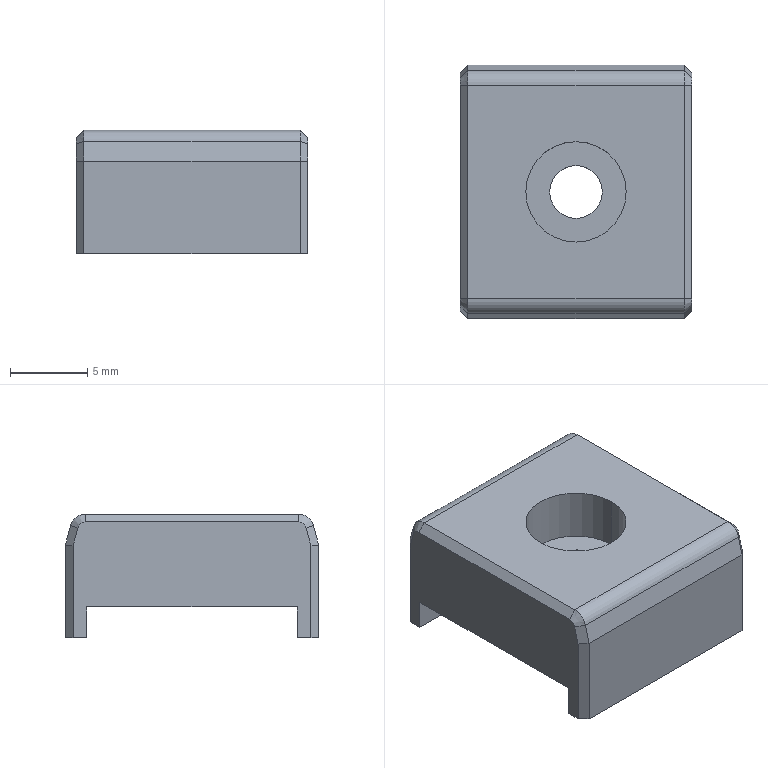Part | SolidWorks | features Chamfer 1, Extrusion 1, HoleWzd 1 | 1 solid | 33 faces | box 15 x 16.4 x 8 mm | volume 1396 mm3 | plane 23 | cylinder 6 | cone 4 | commonest cylinder face diameters 2 x2 3.4 x2 6.5 x2
STEP:
#1=CARTESIAN_POINT('',(-3.25,0.,-3.4));
#2=VERTEX_POINT('',#1);
#3=CARTESIAN_POINT('',(3.25,0.,-3.4));
#4=VERTEX_POINT('',#3);
#5=CARTESIAN_POINT('',(0.,0.,-3.4));
#6=DIRECTION('',(0.,0.,1.));
#7=DIRECTION('',(1.,0.,0.));
#8=AXIS2_PLACEMENT_3D('',#5,#6,#7);
#9=CIRCLE('',#8,3.25);
#10=EDGE_CURVE('',#2,#4,#9,.T.);
#11=ORIENTED_EDGE('',*,*,#10,.F.);
#12=CARTESIAN_POINT('',(-3.25,0.,0.));
#13=VERTEX_POINT('',#12);
#14=CARTESIAN_POINT('',(-3.25,0.,0.));
#15=DIRECTION('',(0.,0.,1.));
#16=VECTOR('',#15,1000.);
#17=LINE('',#14,#16);
#18=EDGE_CURVE('',#2,#13,#17,.T.);
#19=ORIENTED_EDGE('',*,*,#18,.T.);
#20=CARTESIAN_POINT('',(3.25,0.,0.));
#21=VERTEX_POINT('',#20);
#22=CARTESIAN_POINT('',(0.,0.,0.));
#23=DIRECTION('',(0.,0.,1.));
#24=DIRECTION('',(1.,0.,0.));
#25=AXIS2_PLACEMENT_3D('',#22,#23,#24);
#26=CIRCLE('',#25,3.25);
#27=EDGE_CURVE('',#13,#21,#26,.T.);
#28=ORIENTED_EDGE('',*,*,#27,.T.);
#29=CARTESIAN_POINT('',(3.25,0.,0.));
#30=DIRECTION('',(0.,0.,1.));
#31=VECTOR('',#30,1000.);
#32=LINE('',#29,#31);
#33=EDGE_CURVE('',#4,#21,#32,.T.);
#34=ORIENTED_EDGE('',*,*,#33,.F.);
#35=EDGE_LOOP('',(#11,#19,#28,#34));
#36=FACE_OUTER_BOUND('',#35,.T.);
#37=CARTESIAN_POINT('',(0.,0.,0.));
#38=DIRECTION('',(0.,0.,1.));
#39=DIRECTION('',(1.,0.,0.));
#40=AXIS2_PLACEMENT_3D('',#37,#38,#39);
#41=CYLINDRICAL_SURFACE('',#40,3.25);
#42=ADVANCED_FACE('',(#36),#41,.F.);
#43=CARTESIAN_POINT('',(1.7,0.,-6.));
#44=VERTEX_POINT('',#43);
#45=CARTESIAN_POINT('',(-1.7,0.,-6.));
#46=VERTEX_POINT('',#45);
#47=CARTESIAN_POINT('',(0.,0.,-6.));
#48=DIRECTION('',(0.,0.,-1.));
#49=DIRECTION('',(-1.,0.,0.));
#50=AXIS2_PLACEMENT_3D('',#47,#48,#49);
#51=CIRCLE('',#50,1.7);
#52=EDGE_CURVE('',#44,#46,#51,.T.);
#53=ORIENTED_EDGE('',*,*,#52,.T.);
#54=CARTESIAN_POINT('',(-1.7,0.,-3.4));
#55=VERTEX_POINT('',#54);
#56=CARTESIAN_POINT('',(-1.7,0.,0.));
#57=DIRECTION('',(0.,0.,1.));
#58=VECTOR('',#57,1000.);
#59=LINE('',#56,#58);
#60=EDGE_CURVE('',#46,#55,#59,.T.);
#61=ORIENTED_EDGE('',*,*,#60,.T.);
#62=CARTESIAN_POINT('',(1.7,0.,-3.4));
#63=VERTEX_POINT('',#62);
#64=CARTESIAN_POINT('',(0.,0.,-3.4));
#65=DIRECTION('',(0.,0.,1.));
#66=DIRECTION('',(1.,0.,0.));
#67=AXIS2_PLACEMENT_3D('',#64,#65,#66);
#68=CIRCLE('',#67,1.7);
#69=EDGE_CURVE('',#55,#63,#68,.T.);
#70=ORIENTED_EDGE('',*,*,#69,.T.);
#71=CARTESIAN_POINT('',(1.7,0.,0.));
#72=DIRECTION('',(0.,0.,1.));
#73=VECTOR('',#72,1000.);
#74=LINE('',#71,#73);
#75=EDGE_CURVE('',#44,#63,#74,.T.);
#76=ORIENTED_EDGE('',*,*,#75,.F.);
#77=EDGE_LOOP('',(#53,#61,#70,#76));
#78=FACE_OUTER_BOUND('',#77,.T.);
#79=CARTESIAN_POINT('',(0.,0.,0.));
#80=DIRECTION('',(0.,0.,1.));
#81=DIRECTION('',(1.,0.,0.));
#82=AXIS2_PLACEMENT_3D('',#79,#80,#81);
#83=CYLINDRICAL_SURFACE('',#82,1.7);
#84=ADVANCED_FACE('',(#78),#83,.F.);
#85=ORIENTED_EDGE('',*,*,#52,.F.);
#86=CARTESIAN_POINT('',(0.,0.,-6.));
#87=DIRECTION('',(0.,0.,-1.));
#88=DIRECTION('',(-1.,0.,0.));
#89=AXIS2_PLACEMENT_3D('',#86,#87,#88);
#90=CIRCLE('',#89,1.7);
#91=EDGE_CURVE('',#46,#44,#90,.T.);
#92=ORIENTED_EDGE('',*,*,#91,.F.);
#93=EDGE_LOOP('',(#85,#92));
#94=FACE_BOUND('',#93,.T.);
#95=CARTESIAN_POINT('',(7.5,-6.8,-6.));
#96=VERTEX_POINT('',#95);
#97=CARTESIAN_POINT('',(7.5,6.8,-6.));
#98=VERTEX_POINT('',#97);
#99=CARTESIAN_POINT('',(7.5,6.8,-6.));
#100=DIRECTION('',(0.,1.,0.));
#101=VECTOR('',#100,1000.);
#102=LINE('',#99,#101);
#103=EDGE_CURVE('',#96,#98,#102,.T.);
#104=ORIENTED_EDGE('',*,*,#103,.F.);
#105=CARTESIAN_POINT('',(-7.5,-6.8,-6.));
#106=VERTEX_POINT('',#105);
#107=CARTESIAN_POINT('',(25.747,-6.8,-6.));
#108=DIRECTION('',(-1.,0.,0.));
#109=VECTOR('',#108,1000.);
#110=LINE('',#107,#109);
#111=EDGE_CURVE('',#96,#106,#110,.T.);
#112=ORIENTED_EDGE('',*,*,#111,.T.);
#113=CARTESIAN_POINT('',(-7.5,6.8,-6.));
#114=VERTEX_POINT('',#113);
#115=CARTESIAN_POINT('',(-7.5,6.8,-6.));
#116=DIRECTION('',(0.,-1.,0.));
#117=VECTOR('',#116,1000.);
#118=LINE('',#115,#117);
#119=EDGE_CURVE('',#114,#106,#118,.T.);
#120=ORIENTED_EDGE('',*,*,#119,.F.);
#121=CARTESIAN_POINT('',(25.747,6.8,-6.));
#122=DIRECTION('',(-1.,0.,0.));
#123=VECTOR('',#122,1000.);
#124=LINE('',#121,#123);
#125=EDGE_CURVE('',#98,#114,#124,.T.);
#126=ORIENTED_EDGE('',*,*,#125,.F.);
#127=EDGE_LOOP('',(#104,#112,#120,#126));
#128=FACE_OUTER_BOUND('',#127,.T.);
#129=CARTESIAN_POINT('',(25.747,6.8,-6.));
#130=DIRECTION('',(0.,0.,-1.));
#131=DIRECTION('',(-1.,0.,0.));
#132=AXIS2_PLACEMENT_3D('',#129,#130,#131);
#133=PLANE('',#132);
#134=ADVANCED_FACE('',(#94,#128),#133,.T.);
#135=CARTESIAN_POINT('',(7.5,6.8,-8.));
#136=VERTEX_POINT('',#135);
#137=CARTESIAN_POINT('',(7.5,6.8,-6.));
#138=DIRECTION('',(0.,0.,-1.));
#139=VECTOR('',#138,1000.);
#140=LINE('',#137,#139);
#141=EDGE_CURVE('',#98,#136,#140,.T.);
#142=ORIENTED_EDGE('',*,*,#141,.F.);
#143=ORIENTED_EDGE('',*,*,#125,.T.);
#144=CARTESIAN_POINT('',(-7.5,6.8,-8.));
#145=VERTEX_POINT('',#144);
#146=CARTESIAN_POINT('',(-7.5,6.8,-6.));
#147=DIRECTION('',(0.,0.,1.));
#148=VECTOR('',#147,1000.);
#149=LINE('',#146,#148);
#150=EDGE_CURVE('',#145,#114,#149,.T.);
#151=ORIENTED_EDGE('',*,*,#150,.F.);
#152=CARTESIAN_POINT('',(25.747,6.8,-8.));
#153=DIRECTION('',(-1.,0.,0.));
#154=VECTOR('',#153,1000.);
#155=LINE('',#152,#154);
#156=EDGE_CURVE('',#136,#145,#155,.T.);
#157=ORIENTED_EDGE('',*,*,#156,.F.);
#158=EDGE_LOOP('',(#142,#143,#151,#157));
#159=FACE_OUTER_BOUND('',#158,.T.);
#160=CARTESIAN_POINT('',(25.747,6.8,-6.));
#161=DIRECTION('',(0.,-1.,0.));
#162=DIRECTION('',(0.,0.,-1.));
#163=AXIS2_PLACEMENT_3D('',#160,#161,#162);
#164=PLANE('',#163);
#165=ADVANCED_FACE('',(#159),#164,.T.);
#166=CARTESIAN_POINT('',(-7.5,7.7,-8.));
#167=VERTEX_POINT('',#166);
#168=CARTESIAN_POINT('',(-7.5,6.8,-8.));
#169=DIRECTION('',(0.,-1.,0.));
#170=VECTOR('',#169,1000.);
#171=LINE('',#168,#170);
#172=EDGE_CURVE('',#167,#145,#171,.T.);
#173=ORIENTED_EDGE('',*,*,#172,.F.);
#174=CARTESIAN_POINT('',(-7.,8.2,-8.));
#175=VERTEX_POINT('',#174);
#176=CARTESIAN_POINT('',(8.674,23.874,-8.));
#177=DIRECTION('',(0.7071,0.7071,0.));
#178=VECTOR('',#177,1000.);
#179=LINE('',#176,#178);
#180=EDGE_CURVE('',#167,#175,#179,.T.);
#181=ORIENTED_EDGE('',*,*,#180,.T.);
#182=CARTESIAN_POINT('',(7.,8.2,-8.));
#183=VERTEX_POINT('',#182);
#184=CARTESIAN_POINT('',(25.747,8.2,-8.));
#185=DIRECTION('',(-1.,0.,0.));
#186=VECTOR('',#185,1000.);
#187=LINE('',#184,#186);
#188=EDGE_CURVE('',#183,#175,#187,.T.);
#189=ORIENTED_EDGE('',*,*,#188,.F.);
#190=CARTESIAN_POINT('',(7.5,7.7,-8.));
#191=VERTEX_POINT('',#190);
#192=CARTESIAN_POINT('',(17.074,-1.874,-8.));
#193=DIRECTION('',(0.7071,-0.7071,0.));
#194=VECTOR('',#193,1000.);
#195=LINE('',#192,#194);
#196=EDGE_CURVE('',#183,#191,#195,.T.);
#197=ORIENTED_EDGE('',*,*,#196,.T.);
#198=CARTESIAN_POINT('',(7.5,6.8,-8.));
#199=DIRECTION('',(0.,1.,0.));
#200=VECTOR('',#199,1000.);
#201=LINE('',#198,#200);
#202=EDGE_CURVE('',#136,#191,#201,.T.);
#203=ORIENTED_EDGE('',*,*,#202,.F.);
#204=ORIENTED_EDGE('',*,*,#156,.T.);
#205=EDGE_LOOP('',(#173,#181,#189,#197,#203,#204));
#206=FACE_OUTER_BOUND('',#205,.T.);
#207=CARTESIAN_POINT('',(25.747,6.8,-8.));
#208=DIRECTION('',(0.,0.,-1.));
#209=DIRECTION('',(-1.,0.,0.));
#210=AXIS2_PLACEMENT_3D('',#207,#208,#209);
#211=PLANE('',#210);
#212=ADVANCED_FACE('',(#206),#211,.T.);
#213=ORIENTED_EDGE('',*,*,#188,.T.);
#214=CARTESIAN_POINT('',(-7.,8.2,-2.));
#215=VERTEX_POINT('',#214);
#216=CARTESIAN_POINT('',(-7.,8.2,-8.));
#217=DIRECTION('',(0.,0.,1.));
#218=VECTOR('',#217,1000.);
#219=LINE('',#216,#218);
#220=EDGE_CURVE('',#175,#215,#219,.T.);
#221=ORIENTED_EDGE('',*,*,#220,.T.);
#222=CARTESIAN_POINT('',(7.,8.2,-2.));
#223=VERTEX_POINT('',#222);
#224=CARTESIAN_POINT('',(25.747,8.2,-2.));
#225=DIRECTION('',(-1.,0.,0.));
#226=VECTOR('',#225,1000.);
#227=LINE('',#224,#226);
#228=EDGE_CURVE('',#223,#215,#227,.T.);
#229=ORIENTED_EDGE('',*,*,#228,.F.);
#230=CARTESIAN_POINT('',(7.,8.2,-8.));
#231=DIRECTION('',(0.,0.,-1.));
#232=VECTOR('',#231,1000.);
#233=LINE('',#230,#232);
#234=EDGE_CURVE('',#223,#183,#233,.T.);
#235=ORIENTED_EDGE('',*,*,#234,.T.);
#236=EDGE_LOOP('',(#213,#221,#229,#235));
#237=FACE_OUTER_BOUND('',#236,.T.);
#238=CARTESIAN_POINT('',(25.747,8.2,-8.));
#239=DIRECTION('',(0.,1.,0.));
#240=DIRECTION('',(0.,0.,1.));
#241=AXIS2_PLACEMENT_3D('',#238,#239,#240);
#242=PLANE('',#241);
#243=ADVANCED_FACE('',(#237),#242,.T.);
#244=ORIENTED_EDGE('',*,*,#228,.T.);
#245=CARTESIAN_POINT('',(-7.,7.863,-0.7412));
#246=VERTEX_POINT('',#245);
#247=CARTESIAN_POINT('',(-7.,8.2,-2.));
#248=DIRECTION('',(0.,-0.2588,0.9659));
#249=VECTOR('',#248,1000.);
#250=LINE('',#247,#249);
#251=EDGE_CURVE('',#215,#246,#250,.T.);
#252=ORIENTED_EDGE('',*,*,#251,.T.);
#253=CARTESIAN_POINT('',(7.,7.863,-0.7412));
#254=VERTEX_POINT('',#253);
#255=CARTESIAN_POINT('',(25.747,7.863,-0.7412));
#256=DIRECTION('',(-1.,0.,0.));
#257=VECTOR('',#256,1000.);
#258=LINE('',#255,#257);
#259=EDGE_CURVE('',#254,#246,#258,.T.);
#260=ORIENTED_EDGE('',*,*,#259,.F.);
#261=CARTESIAN_POINT('',(7.,8.2,-2.));
#262=DIRECTION('',(0.,0.2588,-0.9659));
#263=VECTOR('',#262,1000.);
#264=LINE('',#261,#263);
#265=EDGE_CURVE('',#254,#223,#264,.T.);
#266=ORIENTED_EDGE('',*,*,#265,.T.);
#267=EDGE_LOOP('',(#244,#252,#260,#266));
#268=FACE_OUTER_BOUND('',#267,.T.);
#269=CARTESIAN_POINT('',(25.747,8.2,-2.));
#270=DIRECTION('',(0.,0.9659,0.2588));
#271=DIRECTION('',(0.,-0.2588,0.9659));
#272=AXIS2_PLACEMENT_3D('',#269,#270,#271);
#273=PLANE('',#272);
#274=ADVANCED_FACE('',(#268),#273,.T.);
#275=ORIENTED_EDGE('',*,*,#259,.T.);
#276=CARTESIAN_POINT('',(-7.,6.897,0.));
#277=VERTEX_POINT('',#276);
#278=CARTESIAN_POINT('',(-7.,6.897,-1.));
#279=DIRECTION('',(1.,0.,0.));
#280=DIRECTION('',(0.,0.,1.));
#281=AXIS2_PLACEMENT_3D('',#278,#279,#280);
#282=CIRCLE('',#281,1.);
#283=EDGE_CURVE('',#246,#277,#282,.T.);
#284=ORIENTED_EDGE('',*,*,#283,.T.);
#285=CARTESIAN_POINT('',(7.,6.897,0.));
#286=VERTEX_POINT('',#285);
#287=CARTESIAN_POINT('',(25.747,6.897,0.));
#288=DIRECTION('',(-1.,0.,0.));
#289=VECTOR('',#288,1000.);
#290=LINE('',#287,#289);
#291=EDGE_CURVE('',#286,#277,#290,.T.);
#292=ORIENTED_EDGE('',*,*,#291,.F.);
#293=CARTESIAN_POINT('',(7.,6.897,-1.));
#294=DIRECTION('',(-1.,0.,0.));
#295=DIRECTION('',(0.,0.,1.));
#296=AXIS2_PLACEMENT_3D('',#293,#294,#295);
#297=CIRCLE('',#296,1.);
#298=EDGE_CURVE('',#286,#254,#297,.T.);
#299=ORIENTED_EDGE('',*,*,#298,.T.);
#300=EDGE_LOOP('',(#275,#284,#292,#299));
#301=FACE_OUTER_BOUND('',#300,.T.);
#302=CARTESIAN_POINT('',(25.747,6.897,-1.));
#303=DIRECTION('',(-1.,0.,0.));
#304=DIRECTION('',(0.,0.,1.));
#305=AXIS2_PLACEMENT_3D('',#302,#303,#304);
#306=CYLINDRICAL_SURFACE('',#305,1.);
#307=ADVANCED_FACE('',(#301),#306,.T.);
#308=CARTESIAN_POINT('',(0.,0.,0.));
#309=DIRECTION('',(0.,0.,1.));
#310=DIRECTION('',(1.,0.,0.));
#311=AXIS2_PLACEMENT_3D('',#308,#309,#310);
#312=CIRCLE('',#311,3.25);
#313=EDGE_CURVE('',#21,#13,#312,.T.);
#314=ORIENTED_EDGE('',*,*,#313,.F.);
#315=ORIENTED_EDGE('',*,*,#27,.F.);
#316=EDGE_LOOP('',(#314,#315));
#317=FACE_BOUND('',#316,.T.);
#318=ORIENTED_EDGE('',*,*,#291,.T.);
#319=CARTESIAN_POINT('',(-7.,-6.897,0.));
#320=VERTEX_POINT('',#319);
#321=CARTESIAN_POINT('',(-7.,-6.897,0.));
#322=DIRECTION('',(0.,-1.,0.));
#323=VECTOR('',#322,1000.);
#324=LINE('',#321,#323);
#325=EDGE_CURVE('',#277,#320,#324,.T.);
#326=ORIENTED_EDGE('',*,*,#325,.T.);
#327=CARTESIAN_POINT('',(7.,-6.897,0.));
#328=VERTEX_POINT('',#327);
#329=CARTESIAN_POINT('',(25.747,-6.897,0.));
#330=DIRECTION('',(-1.,0.,0.));
#331=VECTOR('',#330,1000.);
#332=LINE('',#329,#331);
#333=EDGE_CURVE('',#328,#320,#332,.T.);
#334=ORIENTED_EDGE('',*,*,#333,.F.);
#335=CARTESIAN_POINT('',(7.,6.897,0.));
#336=DIRECTION('',(0.,1.,0.));
#337=VECTOR('',#336,1000.);
#338=LINE('',#335,#337);
#339=EDGE_CURVE('',#328,#286,#338,.T.);
#340=ORIENTED_EDGE('',*,*,#339,.T.);
#341=EDGE_LOOP('',(#318,#326,#334,#340));
#342=FACE_OUTER_BOUND('',#341,.T.);
#343=CARTESIAN_POINT('',(25.747,-6.897,0.));
#344=DIRECTION('',(0.,0.,1.));
#345=DIRECTION('',(1.,0.,0.));
#346=AXIS2_PLACEMENT_3D('',#343,#344,#345);
#347=PLANE('',#346);
#348=ADVANCED_FACE('',(#317,#342),#347,.T.);
#349=ORIENTED_EDGE('',*,*,#333,.T.);
#350=CARTESIAN_POINT('',(-7.,-7.863,-0.7412));
#351=VERTEX_POINT('',#350);
#352=CARTESIAN_POINT('',(-7.,-6.897,-1.));
#353=DIRECTION('',(1.,0.,0.));
#354=DIRECTION('',(0.,0.,1.));
#355=AXIS2_PLACEMENT_3D('',#352,#353,#354);
#356=CIRCLE('',#355,1.);
#357=EDGE_CURVE('',#320,#351,#356,.T.);
#358=ORIENTED_EDGE('',*,*,#357,.T.);
#359=CARTESIAN_POINT('',(7.,-7.863,-0.7412));
#360=VERTEX_POINT('',#359);
#361=CARTESIAN_POINT('',(25.747,-7.863,-0.7412));
#362=DIRECTION('',(-1.,0.,0.));
#363=VECTOR('',#362,1000.);
#364=LINE('',#361,#363);
#365=EDGE_CURVE('',#360,#351,#364,.T.);
#366=ORIENTED_EDGE('',*,*,#365,.F.);
#367=CARTESIAN_POINT('',(7.,-6.897,-1.));
#368=DIRECTION('',(-1.,0.,0.));
#369=DIRECTION('',(0.,0.,1.));
#370=AXIS2_PLACEMENT_3D('',#367,#368,#369);
#371=CIRCLE('',#370,1.);
#372=EDGE_CURVE('',#360,#328,#371,.T.);
#373=ORIENTED_EDGE('',*,*,#372,.T.);
#374=EDGE_LOOP('',(#349,#358,#366,#373));
#375=FACE_OUTER_BOUND('',#374,.T.);
#376=CARTESIAN_POINT('',(25.747,-6.897,-1.));
#377=DIRECTION('',(-1.,0.,0.));
#378=DIRECTION('',(0.,0.,1.));
#379=AXIS2_PLACEMENT_3D('',#376,#377,#378);
#380=CYLINDRICAL_SURFACE('',#379,1.);
#381=ADVANCED_FACE('',(#375),#380,.T.);
#382=ORIENTED_EDGE('',*,*,#365,.T.);
#383=CARTESIAN_POINT('',(-7.,-8.2,-2.));
#384=VERTEX_POINT('',#383);
#385=CARTESIAN_POINT('',(-7.,-8.2,-2.));
#386=DIRECTION('',(0.,-0.2588,-0.9659));
#387=VECTOR('',#386,1000.);
#388=LINE('',#385,#387);
#389=EDGE_CURVE('',#351,#384,#388,.T.);
#390=ORIENTED_EDGE('',*,*,#389,.T.);
#391=CARTESIAN_POINT('',(7.,-8.2,-2.));
#392=VERTEX_POINT('',#391);
#393=CARTESIAN_POINT('',(25.747,-8.2,-2.));
#394=DIRECTION('',(-1.,0.,0.));
#395=VECTOR('',#394,1000.);
#396=LINE('',#393,#395);
#397=EDGE_CURVE('',#392,#384,#396,.T.);
#398=ORIENTED_EDGE('',*,*,#397,.F.);
#399=CARTESIAN_POINT('',(7.,-7.863,-0.7412));
#400=DIRECTION('',(0.,0.2588,0.9659));
#401=VECTOR('',#400,1000.);
#402=LINE('',#399,#401);
#403=EDGE_CURVE('',#392,#360,#402,.T.);
#404=ORIENTED_EDGE('',*,*,#403,.T.);
#405=EDGE_LOOP('',(#382,#390,#398,#404));
#406=FACE_OUTER_BOUND('',#405,.T.);
#407=CARTESIAN_POINT('',(25.747,-8.2,-2.));
#408=DIRECTION('',(0.,-0.9659,0.2588));
#409=DIRECTION('',(0.,-0.2588,-0.9659));
#410=AXIS2_PLACEMENT_3D('',#407,#408,#409);
#411=PLANE('',#410);
#412=ADVANCED_FACE('',(#406),#411,.T.);
#413=CARTESIAN_POINT('',(7.,-8.2,-8.));
#414=VERTEX_POINT('',#413);
#415=CARTESIAN_POINT('',(-7.,-8.2,-8.));
#416=VERTEX_POINT('',#415);
#417=CARTESIAN_POINT('',(25.747,-8.2,-8.));
#418=DIRECTION('',(-1.,0.,0.));
#419=VECTOR('',#418,1000.);
#420=LINE('',#417,#419);
#421=EDGE_CURVE('',#414,#416,#420,.T.);
#422=ORIENTED_EDGE('',*,*,#421,.F.);
#423=CARTESIAN_POINT('',(7.,-8.2,-2.));
#424=DIRECTION('',(0.,0.,1.));
#425=VECTOR('',#424,1000.);
#426=LINE('',#423,#425);
#427=EDGE_CURVE('',#414,#392,#426,.T.);
#428=ORIENTED_EDGE('',*,*,#427,.T.);
#429=ORIENTED_EDGE('',*,*,#397,.T.);
#430=CARTESIAN_POINT('',(-7.,-8.2,-8.));
#431=DIRECTION('',(0.,0.,-1.));
#432=VECTOR('',#431,1000.);
#433=LINE('',#430,#432);
#434=EDGE_CURVE('',#384,#416,#433,.T.);
#435=ORIENTED_EDGE('',*,*,#434,.T.);
#436=EDGE_LOOP('',(#422,#428,#429,#435));
#437=FACE_OUTER_BOUND('',#436,.T.);
#438=CARTESIAN_POINT('',(25.747,-8.2,-8.));
#439=DIRECTION('',(0.,-1.,0.));
#440=DIRECTION('',(0.,0.,-1.));
#441=AXIS2_PLACEMENT_3D('',#438,#439,#440);
#442=PLANE('',#441);
#443=ADVANCED_FACE('',(#437),#442,.T.);
#444=CARTESIAN_POINT('',(7.5,-7.7,-8.));
#445=VERTEX_POINT('',#444);
#446=CARTESIAN_POINT('',(7.5,-6.8,-8.));
#447=VERTEX_POINT('',#446);
#448=CARTESIAN_POINT('',(7.5,-6.8,-8.));
#449=DIRECTION('',(0.,1.,0.));
#450=VECTOR('',#449,1000.);
#451=LINE('',#448,#450);
#452=EDGE_CURVE('',#445,#447,#451,.T.);
#453=ORIENTED_EDGE('',*,*,#452,.F.);
#454=CARTESIAN_POINT('',(17.074,1.874,-8.));
#455=DIRECTION('',(-0.7071,-0.7071,0.));
#456=VECTOR('',#455,1000.);
#457=LINE('',#454,#456);
#458=EDGE_CURVE('',#445,#414,#457,.T.);
#459=ORIENTED_EDGE('',*,*,#458,.T.);
#460=ORIENTED_EDGE('',*,*,#421,.T.);
#461=CARTESIAN_POINT('',(-7.5,-7.7,-8.));
#462=VERTEX_POINT('',#461);
#463=CARTESIAN_POINT('',(8.674,-23.874,-8.));
#464=DIRECTION('',(-0.7071,0.7071,0.));
#465=VECTOR('',#464,1000.);
#466=LINE('',#463,#465);
#467=EDGE_CURVE('',#416,#462,#466,.T.);
#468=ORIENTED_EDGE('',*,*,#467,.T.);
#469=CARTESIAN_POINT('',(-7.5,-6.8,-8.));
#470=VERTEX_POINT('',#469);
#471=CARTESIAN_POINT('',(-7.5,-6.8,-8.));
#472=DIRECTION('',(0.,-1.,0.));
#473=VECTOR('',#472,1000.);
#474=LINE('',#471,#473);
#475=EDGE_CURVE('',#470,#462,#474,.T.);
#476=ORIENTED_EDGE('',*,*,#475,.F.);
#477=CARTESIAN_POINT('',(25.747,-6.8,-8.));
#478=DIRECTION('',(-1.,0.,0.));
#479=VECTOR('',#478,1000.);
#480=LINE('',#477,#479);
#481=EDGE_CURVE('',#447,#470,#480,.T.);
#482=ORIENTED_EDGE('',*,*,#481,.F.);
#483=EDGE_LOOP('',(#453,#459,#460,#468,#476,#482));
#484=FACE_OUTER_BOUND('',#483,.T.);
#485=CARTESIAN_POINT('',(25.747,-6.8,-8.));
#486=DIRECTION('',(0.,0.,-1.));
#487=DIRECTION('',(-1.,0.,0.));
#488=AXIS2_PLACEMENT_3D('',#485,#486,#487);
#489=PLANE('',#488);
#490=ADVANCED_FACE('',(#484),#489,.T.);
#491=CARTESIAN_POINT('',(7.5,-6.8,-6.));
#492=DIRECTION('',(0.,0.,1.));
#493=VECTOR('',#492,1000.);
#494=LINE('',#491,#493);
#495=EDGE_CURVE('',#447,#96,#494,.T.);
#496=ORIENTED_EDGE('',*,*,#495,.F.);
#497=ORIENTED_EDGE('',*,*,#481,.T.);
#498=CARTESIAN_POINT('',(-7.5,-6.8,-6.));
#499=DIRECTION('',(0.,0.,-1.));
#500=VECTOR('',#499,1000.);
#501=LINE('',#498,#500);
#502=EDGE_CURVE('',#106,#470,#501,.T.);
#503=ORIENTED_EDGE('',*,*,#502,.F.);
#504=ORIENTED_EDGE('',*,*,#111,.F.);
#505=EDGE_LOOP('',(#496,#497,#503,#504));
#506=FACE_OUTER_BOUND('',#505,.T.);
#507=CARTESIAN_POINT('',(25.747,-6.8,-6.));
#508=DIRECTION('',(0.,1.,0.));
#509=DIRECTION('',(0.,0.,1.));
#510=AXIS2_PLACEMENT_3D('',#507,#508,#509);
#511=PLANE('',#510);
#512=ADVANCED_FACE('',(#506),#511,.T.);
#513=CARTESIAN_POINT('',(-7.5,7.38,-0.8706));
#514=VERTEX_POINT('',#513);
#515=CARTESIAN_POINT('',(-7.5,7.7,-2.066));
#516=VERTEX_POINT('',#515);
#517=CARTESIAN_POINT('',(-7.5,6.456,2.578));
#518=DIRECTION('',(0.,0.2588,-0.9659));
#519=VECTOR('',#518,1000.);
#520=LINE('',#517,#519);
#521=EDGE_CURVE('',#514,#516,#520,.T.);
#522=ORIENTED_EDGE('',*,*,#521,.T.);
#523=CARTESIAN_POINT('',(-7.5,7.7,-1.));
#524=DIRECTION('',(0.,0.,-1.));
#525=VECTOR('',#524,1000.);
#526=LINE('',#523,#525);
#527=EDGE_CURVE('',#516,#167,#526,.T.);
#528=ORIENTED_EDGE('',*,*,#527,.T.);
#529=ORIENTED_EDGE('',*,*,#172,.T.);
#530=ORIENTED_EDGE('',*,*,#150,.T.);
#531=ORIENTED_EDGE('',*,*,#119,.T.);
#532=ORIENTED_EDGE('',*,*,#502,.T.);
#533=ORIENTED_EDGE('',*,*,#475,.T.);
#534=CARTESIAN_POINT('',(-7.5,-7.7,-2.066));
#535=VERTEX_POINT('',#534);
#536=CARTESIAN_POINT('',(-7.5,-7.7,-1.));
#537=DIRECTION('',(0.,0.,1.));
#538=VECTOR('',#537,1000.);
#539=LINE('',#536,#538);
#540=EDGE_CURVE('',#462,#535,#539,.T.);
#541=ORIENTED_EDGE('',*,*,#540,.T.);
#542=CARTESIAN_POINT('',(-7.5,-7.38,-0.8706));
#543=VERTEX_POINT('',#542);
#544=CARTESIAN_POINT('',(-7.5,-7.38,-0.8706));
#545=DIRECTION('',(0.,0.2588,0.9659));
#546=VECTOR('',#545,1000.);
#547=LINE('',#544,#546);
#548=EDGE_CURVE('',#535,#543,#547,.T.);
#549=ORIENTED_EDGE('',*,*,#548,.T.);
#550=CARTESIAN_POINT('',(-7.5,-6.897,-0.5));
#551=VERTEX_POINT('',#550);
#552=CARTESIAN_POINT('',(-7.5,-6.897,-1.));
#553=DIRECTION('',(-1.,0.,0.));
#554=DIRECTION('',(0.,0.,1.));
#555=AXIS2_PLACEMENT_3D('',#552,#553,#554);
#556=CIRCLE('',#555,0.5);
#557=EDGE_CURVE('',#543,#551,#556,.T.);
#558=ORIENTED_EDGE('',*,*,#557,.T.);
#559=CARTESIAN_POINT('',(-7.5,6.897,-0.5));
#560=VERTEX_POINT('',#559);
#561=CARTESIAN_POINT('',(-7.5,-6.897,-0.5));
#562=DIRECTION('',(0.,1.,0.));
#563=VECTOR('',#562,1000.);
#564=LINE('',#561,#563);
#565=EDGE_CURVE('',#551,#560,#564,.T.);
#566=ORIENTED_EDGE('',*,*,#565,.T.);
#567=CARTESIAN_POINT('',(-7.5,6.897,-1.));
#568=DIRECTION('',(-1.,0.,0.));
#569=DIRECTION('',(0.,0.,1.));
#570=AXIS2_PLACEMENT_3D('',#567,#568,#569);
#571=CIRCLE('',#570,0.5);
#572=EDGE_CURVE('',#560,#514,#571,.T.);
#573=ORIENTED_EDGE('',*,*,#572,.T.);
#574=EDGE_LOOP('',(#522,#528,#529,#530,#531,#532,#533,#541,#549,#558,#566,#573));
#575=FACE_OUTER_BOUND('',#574,.T.);
#576=CARTESIAN_POINT('',(-7.5,-6.897,-1.));
#577=DIRECTION('',(-1.,0.,0.));
#578=DIRECTION('',(0.,0.,1.));
#579=AXIS2_PLACEMENT_3D('',#576,#577,#578);
#580=PLANE('',#579);
#581=ADVANCED_FACE('',(#575),#580,.T.);
#582=ORIENTED_EDGE('',*,*,#202,.T.);
#583=CARTESIAN_POINT('',(7.5,7.7,-2.066));
#584=VERTEX_POINT('',#583);
#585=CARTESIAN_POINT('',(7.5,7.7,-2.));
#586=DIRECTION('',(0.,0.,1.));
#587=VECTOR('',#586,1000.);
#588=LINE('',#585,#587);
#589=EDGE_CURVE('',#191,#584,#588,.T.);
#590=ORIENTED_EDGE('',*,*,#589,.T.);
#591=CARTESIAN_POINT('',(7.5,7.38,-0.8706));
#592=VERTEX_POINT('',#591);
#593=CARTESIAN_POINT('',(7.5,7.38,-0.8706));
#594=DIRECTION('',(0.,-0.2588,0.9659));
#595=VECTOR('',#594,1000.);
#596=LINE('',#593,#595);
#597=EDGE_CURVE('',#584,#592,#596,.T.);
#598=ORIENTED_EDGE('',*,*,#597,.T.);
#599=CARTESIAN_POINT('',(7.5,6.897,-0.5));
#600=VERTEX_POINT('',#599);
#601=CARTESIAN_POINT('',(7.5,6.897,-1.));
#602=DIRECTION('',(1.,0.,0.));
#603=DIRECTION('',(0.,0.,1.));
#604=AXIS2_PLACEMENT_3D('',#601,#602,#603);
#605=CIRCLE('',#604,0.5);
#606=EDGE_CURVE('',#592,#600,#605,.T.);
#607=ORIENTED_EDGE('',*,*,#606,.T.);
#608=CARTESIAN_POINT('',(7.5,-6.897,-0.5));
#609=VERTEX_POINT('',#608);
#610=CARTESIAN_POINT('',(7.5,-6.897,-0.5));
#611=DIRECTION('',(0.,-1.,0.));
#612=VECTOR('',#611,1000.);
#613=LINE('',#610,#612);
#614=EDGE_CURVE('',#600,#609,#613,.T.);
#615=ORIENTED_EDGE('',*,*,#614,.T.);
#616=CARTESIAN_POINT('',(7.5,-7.38,-0.8706));
#617=VERTEX_POINT('',#616);
#618=CARTESIAN_POINT('',(7.5,-6.897,-1.));
#619=DIRECTION('',(1.,0.,0.));
#620=DIRECTION('',(0.,0.,1.));
#621=AXIS2_PLACEMENT_3D('',#618,#619,#620);
#622=CIRCLE('',#621,0.5);
#623=EDGE_CURVE('',#609,#617,#622,.T.);
#624=ORIENTED_EDGE('',*,*,#623,.T.);
#625=CARTESIAN_POINT('',(7.5,-7.7,-2.066));
#626=VERTEX_POINT('',#625);
#627=CARTESIAN_POINT('',(7.5,-7.717,-2.129));
#628=DIRECTION('',(0.,-0.2588,-0.9659));
#629=VECTOR('',#628,1000.);
#630=LINE('',#627,#629);
#631=EDGE_CURVE('',#617,#626,#630,.T.);
#632=ORIENTED_EDGE('',*,*,#631,.T.);
#633=CARTESIAN_POINT('',(7.5,-7.7,-8.));
#634=DIRECTION('',(0.,0.,-1.));
#635=VECTOR('',#634,1000.);
#636=LINE('',#633,#635);
#637=EDGE_CURVE('',#626,#445,#636,.T.);
#638=ORIENTED_EDGE('',*,*,#637,.T.);
#639=ORIENTED_EDGE('',*,*,#452,.T.);
#640=ORIENTED_EDGE('',*,*,#495,.T.);
#641=ORIENTED_EDGE('',*,*,#103,.T.);
#642=ORIENTED_EDGE('',*,*,#141,.T.);
#643=EDGE_LOOP('',(#582,#590,#598,#607,#615,#624,#632,#638,#639,#640,#641,#642));
#644=FACE_OUTER_BOUND('',#643,.T.);
#645=CARTESIAN_POINT('',(7.5,-8.2,-6.));
#646=DIRECTION('',(-1.,0.,0.));
#647=DIRECTION('',(0.,1.,0.));
#648=AXIS2_PLACEMENT_3D('',#645,#646,#647);
#649=PLANE('',#648);
#650=ADVANCED_FACE('',(#644),#649,.F.);
#651=ORIENTED_EDGE('',*,*,#467,.F.);
#652=ORIENTED_EDGE('',*,*,#434,.F.);
#653=CARTESIAN_POINT('',(-7.581,-7.619,-2.076));
#654=DIRECTION('',(0.7041,-0.7041,0.09269));
#655=VECTOR('',#654,1000.);
#656=LINE('',#653,#655);
#657=EDGE_CURVE('',#535,#384,#656,.T.);
#658=ORIENTED_EDGE('',*,*,#657,.F.);
#659=ORIENTED_EDGE('',*,*,#540,.F.);
#660=EDGE_LOOP('',(#651,#652,#658,#659));
#661=FACE_OUTER_BOUND('',#660,.T.);
#662=CARTESIAN_POINT('',(-7.5,-7.7,-1.));
#663=DIRECTION('',(0.7071,0.7071,0.));
#664=DIRECTION('',(0.,0.,1.));
#665=AXIS2_PLACEMENT_3D('',#662,#663,#664);
#666=PLANE('',#665);
#667=ADVANCED_FACE('',(#661),#666,.F.);
#668=ORIENTED_EDGE('',*,*,#657,.T.);
#669=ORIENTED_EDGE('',*,*,#389,.F.);
#670=CARTESIAN_POINT('',(-7.5,-7.38,-0.8706));
#671=DIRECTION('',(0.7071,-0.683,0.183));
#672=VECTOR('',#671,1000.);
#673=LINE('',#670,#672);
#674=EDGE_CURVE('',#543,#351,#673,.T.);
#675=ORIENTED_EDGE('',*,*,#674,.F.);
#676=ORIENTED_EDGE('',*,*,#548,.F.);
#677=EDGE_LOOP('',(#668,#669,#675,#676));
#678=FACE_OUTER_BOUND('',#677,.T.);
#679=CARTESIAN_POINT('',(-7.5,-7.38,-0.8706));
#680=DIRECTION('',(0.7071,0.683,-0.183));
#681=DIRECTION('',(0.,0.2588,0.9659));
#682=AXIS2_PLACEMENT_3D('',#679,#680,#681);
#683=PLANE('',#682);
#684=ADVANCED_FACE('',(#678),#683,.F.);
#685=ORIENTED_EDGE('',*,*,#674,.T.);
#686=ORIENTED_EDGE('',*,*,#357,.F.);
#687=CARTESIAN_POINT('',(-7.5,-6.897,-0.5));
#688=DIRECTION('',(0.7071,0.,0.7071));
#689=VECTOR('',#688,1000.);
#690=LINE('',#687,#689);
#691=EDGE_CURVE('',#551,#320,#690,.T.);
#692=ORIENTED_EDGE('',*,*,#691,.F.);
#693=ORIENTED_EDGE('',*,*,#557,.F.);
#694=EDGE_LOOP('',(#685,#686,#692,#693));
#695=FACE_OUTER_BOUND('',#694,.T.);
#696=CARTESIAN_POINT('',(-7.5,-6.897,-1.));
#697=DIRECTION('',(1.,0.,0.));
#698=DIRECTION('',(0.,0.,-1.));
#699=AXIS2_PLACEMENT_3D('',#696,#697,#698);
#700=CONICAL_SURFACE('',#699,0.5,0.7854);
#701=ADVANCED_FACE('',(#695),#700,.T.);
#702=ORIENTED_EDGE('',*,*,#691,.T.);
#703=ORIENTED_EDGE('',*,*,#325,.F.);
#704=CARTESIAN_POINT('',(-7.5,6.897,-0.5));
#705=DIRECTION('',(0.7071,0.,0.7071));
#706=VECTOR('',#705,1000.);
#707=LINE('',#704,#706);
#708=EDGE_CURVE('',#560,#277,#707,.T.);
#709=ORIENTED_EDGE('',*,*,#708,.F.);
#710=ORIENTED_EDGE('',*,*,#565,.F.);
#711=EDGE_LOOP('',(#702,#703,#709,#710));
#712=FACE_OUTER_BOUND('',#711,.T.);
#713=CARTESIAN_POINT('',(-7.5,-6.897,-0.5));
#714=DIRECTION('',(0.7071,0.,-0.7071));
#715=DIRECTION('',(0.,1.,0.));
#716=AXIS2_PLACEMENT_3D('',#713,#714,#715);
#717=PLANE('',#716);
#718=ADVANCED_FACE('',(#712),#717,.F.);
#719=ORIENTED_EDGE('',*,*,#708,.T.);
#720=ORIENTED_EDGE('',*,*,#283,.F.);
#721=CARTESIAN_POINT('',(-7.5,7.38,-0.8706));
#722=DIRECTION('',(0.7071,0.683,0.183));
#723=VECTOR('',#722,1000.);
#724=LINE('',#721,#723);
#725=EDGE_CURVE('',#514,#246,#724,.T.);
#726=ORIENTED_EDGE('',*,*,#725,.F.);
#727=ORIENTED_EDGE('',*,*,#572,.F.);
#728=EDGE_LOOP('',(#719,#720,#726,#727));
#729=FACE_OUTER_BOUND('',#728,.T.);
#730=CARTESIAN_POINT('',(-7.5,6.897,-1.));
#731=DIRECTION('',(1.,0.,0.));
#732=DIRECTION('',(0.,0.,-1.));
#733=AXIS2_PLACEMENT_3D('',#730,#731,#732);
#734=CONICAL_SURFACE('',#733,0.5,0.7854);
#735=ADVANCED_FACE('',(#729),#734,.T.);
#736=ORIENTED_EDGE('',*,*,#725,.T.);
#737=ORIENTED_EDGE('',*,*,#251,.F.);
#738=CARTESIAN_POINT('',(-7.814,7.386,-2.107));
#739=DIRECTION('',(0.7041,0.7041,0.09269));
#740=VECTOR('',#739,1000.);
#741=LINE('',#738,#740);
#742=EDGE_CURVE('',#516,#215,#741,.T.);
#743=ORIENTED_EDGE('',*,*,#742,.F.);
#744=ORIENTED_EDGE('',*,*,#521,.F.);
#745=EDGE_LOOP('',(#736,#737,#743,#744));
#746=FACE_OUTER_BOUND('',#745,.T.);
#747=CARTESIAN_POINT('',(-7.5,6.456,2.578));
#748=DIRECTION('',(0.7071,-0.683,-0.183));
#749=DIRECTION('',(0.,0.2588,-0.9659));
#750=AXIS2_PLACEMENT_3D('',#747,#748,#749);
#751=PLANE('',#750);
#752=ADVANCED_FACE('',(#746),#751,.F.);
#753=ORIENTED_EDGE('',*,*,#742,.T.);
#754=ORIENTED_EDGE('',*,*,#220,.F.);
#755=ORIENTED_EDGE('',*,*,#180,.F.);
#756=ORIENTED_EDGE('',*,*,#527,.F.);
#757=EDGE_LOOP('',(#753,#754,#755,#756));
#758=FACE_OUTER_BOUND('',#757,.T.);
#759=CARTESIAN_POINT('',(-7.5,7.7,-1.));
#760=DIRECTION('',(0.7071,-0.7071,0.));
#761=DIRECTION('',(0.,0.,-1.));
#762=AXIS2_PLACEMENT_3D('',#759,#760,#761);
#763=PLANE('',#762);
#764=ADVANCED_FACE('',(#758),#763,.F.);
#765=ORIENTED_EDGE('',*,*,#458,.F.);
#766=ORIENTED_EDGE('',*,*,#637,.F.);
#767=CARTESIAN_POINT('',(7.244,-7.956,-2.032));
#768=DIRECTION('',(0.7041,0.7041,-0.09269));
#769=VECTOR('',#768,1000.);
#770=LINE('',#767,#769);
#771=EDGE_CURVE('',#392,#626,#770,.T.);
#772=ORIENTED_EDGE('',*,*,#771,.F.);
#773=ORIENTED_EDGE('',*,*,#427,.F.);
#774=EDGE_LOOP('',(#765,#766,#772,#773));
#775=FACE_OUTER_BOUND('',#774,.T.);
#776=CARTESIAN_POINT('',(7.5,-7.7,-6.));
#777=DIRECTION('',(0.7071,-0.7071,0.));
#778=DIRECTION('',(0.,0.,1.));
#779=AXIS2_PLACEMENT_3D('',#776,#777,#778);
#780=PLANE('',#779);
#781=ADVANCED_FACE('',(#775),#780,.T.);
#782=ORIENTED_EDGE('',*,*,#771,.T.);
#783=ORIENTED_EDGE('',*,*,#631,.F.);
#784=CARTESIAN_POINT('',(7.,-7.863,-0.7412));
#785=DIRECTION('',(0.7071,0.683,-0.183));
#786=VECTOR('',#785,1000.);
#787=LINE('',#784,#786);
#788=EDGE_CURVE('',#360,#617,#787,.T.);
#789=ORIENTED_EDGE('',*,*,#788,.F.);
#790=ORIENTED_EDGE('',*,*,#403,.F.);
#791=EDGE_LOOP('',(#782,#783,#789,#790));
#792=FACE_OUTER_BOUND('',#791,.T.);
#793=CARTESIAN_POINT('',(7.5,-8.717,-5.861));
#794=DIRECTION('',(0.7071,-0.683,0.183));
#795=DIRECTION('',(0.,0.2588,0.9659));
#796=AXIS2_PLACEMENT_3D('',#793,#794,#795);
#797=PLANE('',#796);
#798=ADVANCED_FACE('',(#792),#797,.T.);
#799=ORIENTED_EDGE('',*,*,#788,.T.);
#800=ORIENTED_EDGE('',*,*,#623,.F.);
#801=CARTESIAN_POINT('',(7.,-6.897,0.));
#802=DIRECTION('',(0.7071,0.,-0.7071));
#803=VECTOR('',#802,1000.);
#804=LINE('',#801,#803);
#805=EDGE_CURVE('',#328,#609,#804,.T.);
#806=ORIENTED_EDGE('',*,*,#805,.F.);
#807=ORIENTED_EDGE('',*,*,#372,.F.);
#808=EDGE_LOOP('',(#799,#800,#806,#807));
#809=FACE_OUTER_BOUND('',#808,.T.);
#810=CARTESIAN_POINT('',(7.5,-6.897,-1.));
#811=DIRECTION('',(-1.,0.,0.));
#812=DIRECTION('',(0.,0.,1.));
#813=AXIS2_PLACEMENT_3D('',#810,#811,#812);
#814=CONICAL_SURFACE('',#813,0.5,0.7854);
#815=ADVANCED_FACE('',(#809),#814,.T.);
#816=ORIENTED_EDGE('',*,*,#805,.T.);
#817=ORIENTED_EDGE('',*,*,#614,.F.);
#818=CARTESIAN_POINT('',(7.,6.897,0.));
#819=DIRECTION('',(0.7071,0.,-0.7071));
#820=VECTOR('',#819,1000.);
#821=LINE('',#818,#820);
#822=EDGE_CURVE('',#286,#600,#821,.T.);
#823=ORIENTED_EDGE('',*,*,#822,.F.);
#824=ORIENTED_EDGE('',*,*,#339,.F.);
#825=EDGE_LOOP('',(#816,#817,#823,#824));
#826=FACE_OUTER_BOUND('',#825,.T.);
#827=CARTESIAN_POINT('',(7.5,-8.2,-0.5));
#828=DIRECTION('',(0.7071,0.,0.7071));
#829=DIRECTION('',(0.,1.,0.));
#830=AXIS2_PLACEMENT_3D('',#827,#828,#829);
#831=PLANE('',#830);
#832=ADVANCED_FACE('',(#826),#831,.T.);
#833=ORIENTED_EDGE('',*,*,#822,.T.);
#834=ORIENTED_EDGE('',*,*,#606,.F.);
#835=CARTESIAN_POINT('',(7.,7.863,-0.7412));
#836=DIRECTION('',(0.7071,-0.683,-0.183));
#837=VECTOR('',#836,1000.);
#838=LINE('',#835,#837);
#839=EDGE_CURVE('',#254,#592,#838,.T.);
#840=ORIENTED_EDGE('',*,*,#839,.F.);
#841=ORIENTED_EDGE('',*,*,#298,.F.);
#842=EDGE_LOOP('',(#833,#834,#840,#841));
#843=FACE_OUTER_BOUND('',#842,.T.);
#844=CARTESIAN_POINT('',(7.5,6.897,-1.));
#845=DIRECTION('',(-1.,0.,0.));
#846=DIRECTION('',(0.,0.,1.));
#847=AXIS2_PLACEMENT_3D('',#844,#845,#846);
#848=CONICAL_SURFACE('',#847,0.5,0.7854);
#849=ADVANCED_FACE('',(#843),#848,.T.);
#850=ORIENTED_EDGE('',*,*,#839,.T.);
#851=ORIENTED_EDGE('',*,*,#597,.F.);
#852=CARTESIAN_POINT('',(7.521,7.679,-2.069));
#853=DIRECTION('',(0.7041,-0.7041,-0.09269));
#854=VECTOR('',#853,1000.);
#855=LINE('',#852,#854);
#856=EDGE_CURVE('',#223,#584,#855,.T.);
#857=ORIENTED_EDGE('',*,*,#856,.F.);
#858=ORIENTED_EDGE('',*,*,#265,.F.);
#859=EDGE_LOOP('',(#850,#851,#857,#858));
#860=FACE_OUTER_BOUND('',#859,.T.);
#861=CARTESIAN_POINT('',(7.5,7.618,-1.761));
#862=DIRECTION('',(0.7071,0.683,0.183));
#863=DIRECTION('',(0.,0.2588,-0.9659));
#864=AXIS2_PLACEMENT_3D('',#861,#862,#863);
#865=PLANE('',#864);
#866=ADVANCED_FACE('',(#860),#865,.T.);
#867=ORIENTED_EDGE('',*,*,#196,.F.);
#868=ORIENTED_EDGE('',*,*,#234,.F.);
#869=ORIENTED_EDGE('',*,*,#856,.T.);
#870=ORIENTED_EDGE('',*,*,#589,.F.);
#871=EDGE_LOOP('',(#867,#868,#869,#870));
#872=FACE_OUTER_BOUND('',#871,.T.);
#873=CARTESIAN_POINT('',(7.5,7.7,-6.));
#874=DIRECTION('',(0.7071,0.7071,0.));
#875=DIRECTION('',(0.,0.,-1.));
#876=AXIS2_PLACEMENT_3D('',#873,#874,#875);
#877=PLANE('',#876);
#878=ADVANCED_FACE('',(#872),#877,.T.);
#879=ORIENTED_EDGE('',*,*,#60,.F.);
#880=ORIENTED_EDGE('',*,*,#91,.T.);
#881=ORIENTED_EDGE('',*,*,#75,.T.);
#882=CARTESIAN_POINT('',(0.,0.,-3.4));
#883=DIRECTION('',(0.,0.,1.));
#884=DIRECTION('',(1.,0.,0.));
#885=AXIS2_PLACEMENT_3D('',#882,#883,#884);
#886=CIRCLE('',#885,1.7);
#887=EDGE_CURVE('',#63,#55,#886,.T.);
#888=ORIENTED_EDGE('',*,*,#887,.T.);
#889=EDGE_LOOP('',(#879,#880,#881,#888));
#890=FACE_OUTER_BOUND('',#889,.T.);
#891=CARTESIAN_POINT('',(0.,0.,0.));
#892=DIRECTION('',(0.,0.,1.));
#893=DIRECTION('',(1.,0.,0.));
#894=AXIS2_PLACEMENT_3D('',#891,#892,#893);
#895=CYLINDRICAL_SURFACE('',#894,1.7);
#896=ADVANCED_FACE('',(#890),#895,.F.);
#897=ORIENTED_EDGE('',*,*,#887,.F.);
#898=ORIENTED_EDGE('',*,*,#69,.F.);
#899=EDGE_LOOP('',(#897,#898));
#900=FACE_BOUND('',#899,.T.);
#901=CARTESIAN_POINT('',(0.,0.,-3.4));
#902=DIRECTION('',(0.,0.,1.));
#903=DIRECTION('',(1.,0.,0.));
#904=AXIS2_PLACEMENT_3D('',#901,#902,#903);
#905=CIRCLE('',#904,3.25);
#906=EDGE_CURVE('',#4,#2,#905,.T.);
#907=ORIENTED_EDGE('',*,*,#906,.T.);
#908=ORIENTED_EDGE('',*,*,#10,.T.);
#909=EDGE_LOOP('',(#907,#908));
#910=FACE_OUTER_BOUND('',#909,.T.);
#911=CARTESIAN_POINT('',(1.7,0.,-3.4));
#912=DIRECTION('',(0.,0.,-1.));
#913=DIRECTION('',(-1.,0.,0.));
#914=AXIS2_PLACEMENT_3D('',#911,#912,#913);
#915=PLANE('',#914);
#916=ADVANCED_FACE('',(#900,#910),#915,.F.);
#917=ORIENTED_EDGE('',*,*,#18,.F.);
#918=ORIENTED_EDGE('',*,*,#906,.F.);
#919=ORIENTED_EDGE('',*,*,#33,.T.);
#920=ORIENTED_EDGE('',*,*,#313,.T.);
#921=EDGE_LOOP('',(#917,#918,#919,#920));
#922=FACE_OUTER_BOUND('',#921,.T.);
#923=CARTESIAN_POINT('',(0.,0.,0.));
#924=DIRECTION('',(0.,0.,1.));
#925=DIRECTION('',(1.,0.,0.));
#926=AXIS2_PLACEMENT_3D('',#923,#924,#925);
#927=CYLINDRICAL_SURFACE('',#926,3.25);
#928=ADVANCED_FACE('',(#922),#927,.F.);
#929=CLOSED_SHELL('',(#42,#84,#134,#165,#212,#243,#274,#307,#348,#381,#412,#443,#490,#512,#581,#650,#667,#684,#701,#718,#735,#752,#764,#781,#798,#815,#832,#849,#866,#878,#896,#916,#928));
#930=MANIFOLD_SOLID_BREP('',#929);
#931=CARTESIAN_POINT('',(0.,0.,0.));
#932=DIRECTION('',(0.,0.,1.));
#933=DIRECTION('',(1.,0.,0.));
#934=AXIS2_PLACEMENT_3D('',#931,#932,#933);
#935=(LENGTH_UNIT()NAMED_UNIT(*)SI_UNIT(.MILLI.,.METRE.));
#936=UNCERTAINTY_MEASURE_WITH_UNIT(LENGTH_MEASURE(0.00001),#935,'','');
#937=(NAMED_UNIT(*)PLANE_ANGLE_UNIT()SI_UNIT($,.RADIAN.));
#938=(NAMED_UNIT(*)SI_UNIT($,.STERADIAN.)SOLID_ANGLE_UNIT());
#939=(GEOMETRIC_REPRESENTATION_CONTEXT(3)GLOBAL_UNCERTAINTY_ASSIGNED_CONTEXT((#936))GLOBAL_UNIT_ASSIGNED_CONTEXT((#935,#937,#938))REPRESENTATION_CONTEXT('',''));
#940=ADVANCED_BREP_SHAPE_REPRESENTATION('',(#930,#934),#939);